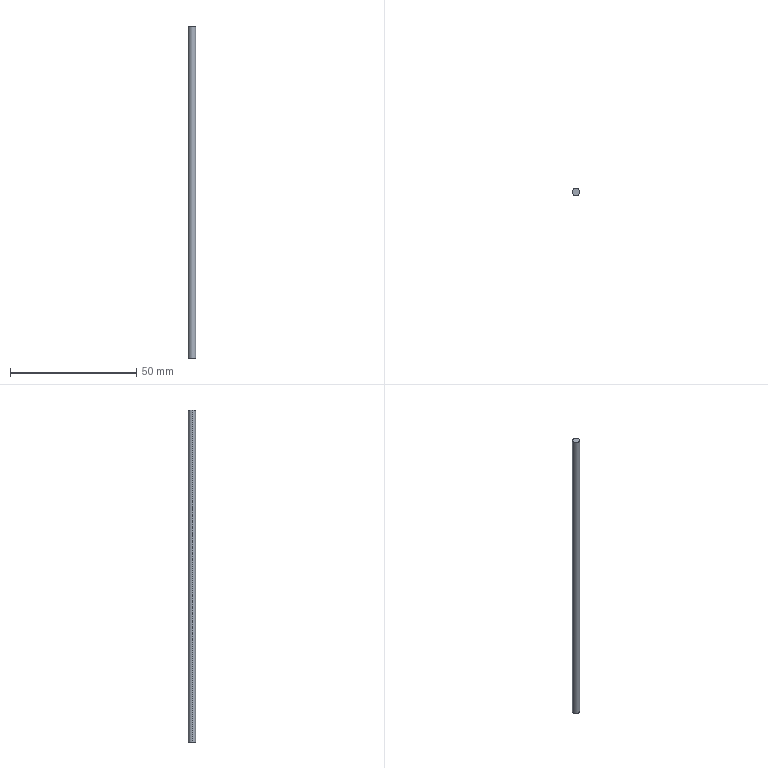Part | SolidWorks | features Extrusion 1 | 1 solid | 4 faces | box 2.88 x 2.88 x 131.6 mm | volume 857.296 mm3 | cylinder 2 | plane 2 | commonest cylinder face diameters 2.88 x2
STEP:
#1=CARTESIAN_POINT('',(1.44,0.,131.6));
#2=VERTEX_POINT('',#1);
#3=CARTESIAN_POINT('',(-1.44,0.,131.6));
#4=VERTEX_POINT('',#3);
#5=CARTESIAN_POINT('',(0.,0.,131.6));
#6=DIRECTION('',(0.,0.,1.));
#7=DIRECTION('',(1.,0.,0.));
#8=AXIS2_PLACEMENT_3D('',#5,#6,#7);
#9=CIRCLE('',#8,1.44);
#10=EDGE_CURVE('',#2,#4,#9,.T.);
#11=ORIENTED_EDGE('',*,*,#10,.F.);
#12=CARTESIAN_POINT('',(1.44,0.,0.));
#13=VERTEX_POINT('',#12);
#14=CARTESIAN_POINT('',(1.44,0.,131.6));
#15=DIRECTION('',(0.,0.,-1.));
#16=VECTOR('',#15,1000.);
#17=LINE('',#14,#16);
#18=EDGE_CURVE('',#2,#13,#17,.T.);
#19=ORIENTED_EDGE('',*,*,#18,.T.);
#20=CARTESIAN_POINT('',(-1.44,0.,0.));
#21=VERTEX_POINT('',#20);
#22=CARTESIAN_POINT('',(0.,0.,0.));
#23=DIRECTION('',(0.,0.,1.));
#24=DIRECTION('',(1.,0.,0.));
#25=AXIS2_PLACEMENT_3D('',#22,#23,#24);
#26=CIRCLE('',#25,1.44);
#27=EDGE_CURVE('',#13,#21,#26,.T.);
#28=ORIENTED_EDGE('',*,*,#27,.T.);
#29=CARTESIAN_POINT('',(-1.44,0.,131.6));
#30=DIRECTION('',(0.,0.,-1.));
#31=VECTOR('',#30,1000.);
#32=LINE('',#29,#31);
#33=EDGE_CURVE('',#4,#21,#32,.T.);
#34=ORIENTED_EDGE('',*,*,#33,.F.);
#35=EDGE_LOOP('',(#11,#19,#28,#34));
#36=FACE_OUTER_BOUND('',#35,.T.);
#37=CARTESIAN_POINT('',(0.,0.,131.6));
#38=DIRECTION('',(0.,0.,-1.));
#39=DIRECTION('',(-1.,0.,0.));
#40=AXIS2_PLACEMENT_3D('',#37,#38,#39);
#41=CYLINDRICAL_SURFACE('',#40,1.44);
#42=ADVANCED_FACE('',(#36),#41,.T.);
#43=ORIENTED_EDGE('',*,*,#18,.F.);
#44=CARTESIAN_POINT('',(0.,0.,131.6));
#45=DIRECTION('',(0.,0.,1.));
#46=DIRECTION('',(1.,0.,0.));
#47=AXIS2_PLACEMENT_3D('',#44,#45,#46);
#48=CIRCLE('',#47,1.44);
#49=EDGE_CURVE('',#4,#2,#48,.T.);
#50=ORIENTED_EDGE('',*,*,#49,.F.);
#51=ORIENTED_EDGE('',*,*,#33,.T.);
#52=CARTESIAN_POINT('',(0.,0.,0.));
#53=DIRECTION('',(0.,0.,1.));
#54=DIRECTION('',(1.,0.,0.));
#55=AXIS2_PLACEMENT_3D('',#52,#53,#54);
#56=CIRCLE('',#55,1.44);
#57=EDGE_CURVE('',#21,#13,#56,.T.);
#58=ORIENTED_EDGE('',*,*,#57,.T.);
#59=EDGE_LOOP('',(#43,#50,#51,#58));
#60=FACE_OUTER_BOUND('',#59,.T.);
#61=CARTESIAN_POINT('',(0.,0.,131.6));
#62=DIRECTION('',(0.,0.,-1.));
#63=DIRECTION('',(-1.,0.,0.));
#64=AXIS2_PLACEMENT_3D('',#61,#62,#63);
#65=CYLINDRICAL_SURFACE('',#64,1.44);
#66=ADVANCED_FACE('',(#60),#65,.T.);
#67=ORIENTED_EDGE('',*,*,#49,.T.);
#68=ORIENTED_EDGE('',*,*,#10,.T.);
#69=EDGE_LOOP('',(#67,#68));
#70=FACE_OUTER_BOUND('',#69,.T.);
#71=CARTESIAN_POINT('',(0.,0.,131.6));
#72=DIRECTION('',(0.,0.,1.));
#73=DIRECTION('',(1.,0.,0.));
#74=AXIS2_PLACEMENT_3D('',#71,#72,#73);
#75=PLANE('',#74);
#76=ADVANCED_FACE('',(#70),#75,.T.);
#77=ORIENTED_EDGE('',*,*,#57,.F.);
#78=ORIENTED_EDGE('',*,*,#27,.F.);
#79=EDGE_LOOP('',(#77,#78));
#80=FACE_OUTER_BOUND('',#79,.T.);
#81=CARTESIAN_POINT('',(0.,0.,0.));
#82=DIRECTION('',(0.,0.,1.));
#83=DIRECTION('',(1.,0.,0.));
#84=AXIS2_PLACEMENT_3D('',#81,#82,#83);
#85=PLANE('',#84);
#86=ADVANCED_FACE('',(#80),#85,.F.);
#87=CLOSED_SHELL('',(#42,#66,#76,#86));
#88=MANIFOLD_SOLID_BREP('',#87);
#89=CARTESIAN_POINT('',(0.,0.,0.));
#90=DIRECTION('',(0.,0.,1.));
#91=DIRECTION('',(1.,0.,0.));
#92=AXIS2_PLACEMENT_3D('',#89,#90,#91);
#93=(LENGTH_UNIT()NAMED_UNIT(*)SI_UNIT(.MILLI.,.METRE.));
#94=UNCERTAINTY_MEASURE_WITH_UNIT(LENGTH_MEASURE(0.00001),#93,'','');
#95=(NAMED_UNIT(*)PLANE_ANGLE_UNIT()SI_UNIT($,.RADIAN.));
#96=(NAMED_UNIT(*)SI_UNIT($,.STERADIAN.)SOLID_ANGLE_UNIT());
#97=(GEOMETRIC_REPRESENTATION_CONTEXT(3)GLOBAL_UNCERTAINTY_ASSIGNED_CONTEXT((#94))GLOBAL_UNIT_ASSIGNED_CONTEXT((#93,#95,#96))REPRESENTATION_CONTEXT('',''));
#98=ADVANCED_BREP_SHAPE_REPRESENTATION('',(#88,#92),#97);